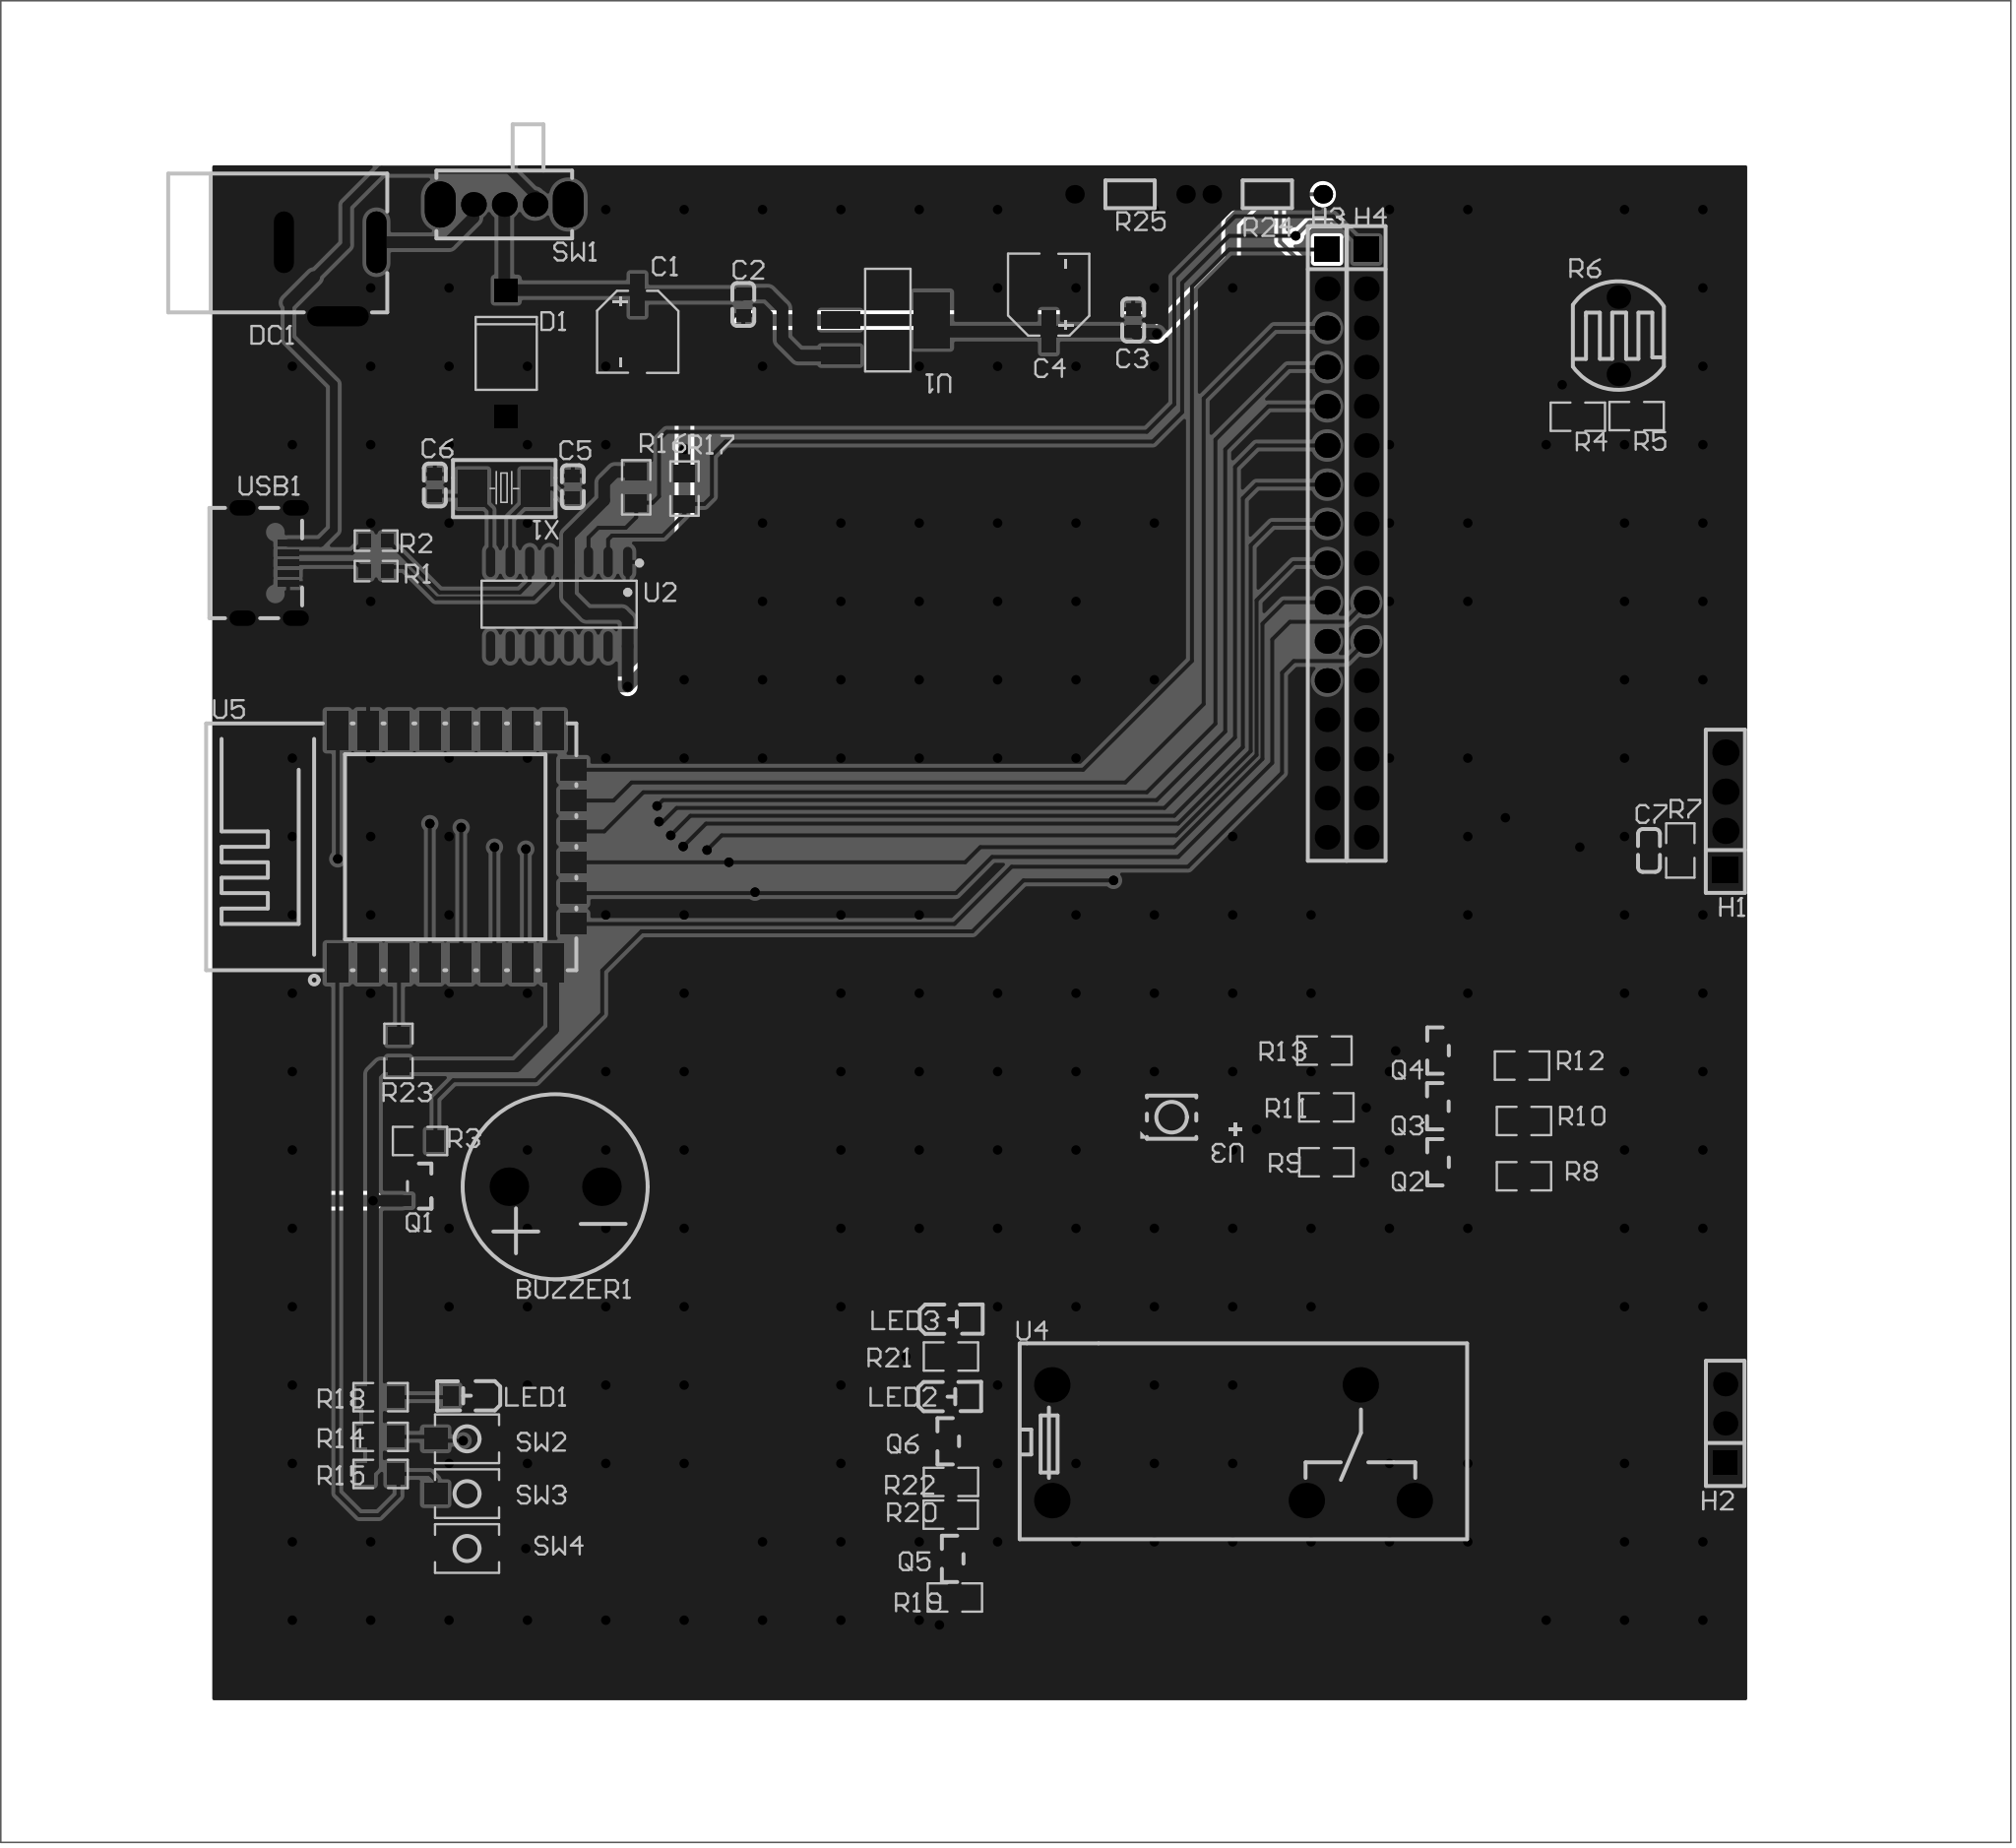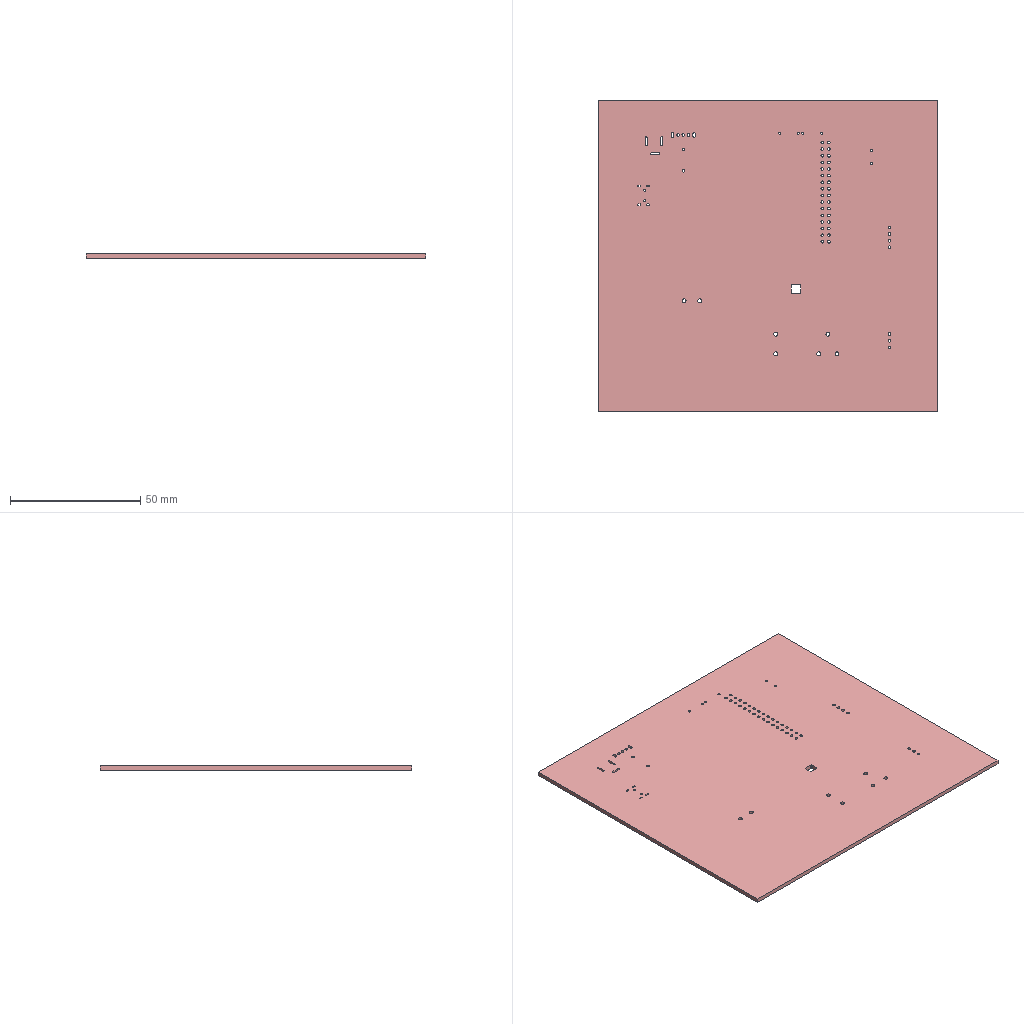Circuit board layout | Altium Designer | box 130.3 x 119.4 x 1.6 mm
Layer stack:
# Altium Designer layer stack of  (unit mm; dielectric type: 0 none, 1 core, 2 prepreg, 3 surface material)
index,name,kind,layer,copper_thickness_mm,dielectric_type,dielectric_thickness_mm,dielectric_material,dielectric_constant
0,Top Paste Mask Layer,other,,,,,,
1,Top Silkscreen Layer,other,,,,,,
2,Top Solder Mask Layer,dielectric,,,3,0.01,,3.3
3,Top Layer,copper,Top Layer,0.035,,,,
4,Dielectric1,dielectric,,,3,1.51,FR4,4.5
5,Bottom Layer,copper,Bottom Layer,0.035,,,,
6,Bottom Solder Mask Layer,dielectric,,,3,0.01,,3.3
7,Bottom Silkscreen Layer,other,,,,,,
8,Bottom Paste Mask Layer,other,,,,,,
# drill layer pairs: low layer,high layer
drill_pair,Top Layer,Bottom Layer
Part placement:
Designator,Comment,Layer,Footprint,Center-X(mm),Center-Y(mm),Rotation
BUZZER1,buzzer,TopLayer,BUZ-TH_BD12.0-P6.00-D0.9-RD,105.788,112.353,180
C1,10uF,TopLayer,C_Ele_SMD_5x5.4mm,111.125,167.767,270
C2,100nF,TopLayer,C0603,117.983,169.545,90
C3,100nF,TopLayer,C0603,143.256,168.529,270
C4,10uF,TopLayer,C_Ele_SMD_5x5.4mm,137.795,170.18,90
C5,22pF,TopLayer,C0603,106.934,157.734,270
C6,22pF,TopLayer,C0603,97.987,157.843,270
C7,100nF,TopLayer,C0603,176.695,134.149,270
D1,SMA_DIODE,TopLayer,SOD-57_BD3.8-L4.6-P9.00-D0.8-RD,102.616,166.37,270
DC1,,TopLayer,DC-2.0,91.204,171.176,180
H1,,TopLayer,HDR-TH_4P-P2.54-V-F,181.648,136.69,90
H2,,TopLayer,HDR-TH_3P-P2.54-V-F,181.637,97.012,90
H3,,TopLayer,HDR-TH_16P-P2.54-V-F,155.829,154.051,270
H4,,TopLayer,HDR-TH_16P-P2.54-V-F,158.369,154.051,270
LED1,,TopLayer,LED_0805,100.126,98.801,180
LED2,,TopLayer,LED_0805,131.423,98.747,0
LED3,,TopLayer,LED_0805,131.522,103.764,0
Q1,,TopLayer,S8550P_SOT,97.113,112.395,180
Q2,,TopLayer,S8050_SOT-23,163.021,113.939,0
Q3,,TopLayer,S8050_SOT-23,163.01,117.571,0
Q4,,TopLayer,S8050_SOT-23,163.021,121.178,0
Q5,,TopLayer,S8050_SOT-23,131.557,88.23,0
Q6,,TopLayer,S8050_SOT-23,131.269,95.85,0
R3,1K,TopLayer,R0805,97.028,115.316,180
R4,10K,TopLayer,R0805,172.083,162.264,0
R5,4.7K,TopLayer,R0805,175.895,162.306,0
R6,GL7528,TopLayer,RES-TH_L7.0-W5.9-P5.00-D0.5,174.711,167.516,0
R7,4.7K,TopLayer,R0805,178.726,134.149,270
R8,1.5K,TopLayer,R0805,168.591,113.031,180
R10,1.5K,TopLayer,R0805,168.591,116.615,180
R12,1.5K,TopLayer,R0805,168.464,120.205,180
R14,10K,TopLayer,R0805,94.472,96.139,0
R15,10K,TopLayer,R0805,94.472,93.734,0
R16,10K,TopLayer,R0805,111.042,157.69,270
R17,10K,TopLayer,R0805,114.173,157.607,270
R18,4.7K,TopLayer,R0805,94.472,98.71,0
R19,1.5K,TopLayer,R0805,131.699,85.725,0
R20,1.5K,TopLayer,R0805,131.43,91.097,0
R21,10K,TopLayer,R0805,131.445,101.346,180
R22,1.5K,TopLayer,R0805,131.445,93.218,0
R23,10K,TopLayer,R0805,95.631,121.158,90
R24,10K,TopLayer,Res_1/8W,151.954,176.686,0
R25,4.7K,TopLayer,Res_1/8W,143.057,176.686,0
SW1,,TopLayer,拨动开关_侧,102.489,176.022,180
SW2,,TopLayer,Key_SMD_3x4x2,100.076,96.012,0
SW3,,TopLayer,Key_SMD_3x4x2,100.076,92.456,0
SW4,,TopLayer,Key_SMD_3x4x2,100.076,88.9,180
U1,AMS1117-3.3,TopLayer,SOT-223-3_L6.5-W3.4-P2.30-LS7.0-BR,127.254,168.529,180
U2,CH340G,TopLayer,SOIC-16_L9.9-W3.9-P1.27-LS6.0-BL,106.045,150.114,180
U3,6028-ZRGBF-SMD-H2,TopLayer,LED-SMD_4P-L3.2-W2.8_ZRGBF-SMD-H2,145.749,116.86,180
U4,SSKD6132,TopLayer,RELAY-TH_G2R-1,149.733,95.758,0
U5,ESP8266,TopLayer,WIFIM-SMD_ESP-12F-ESP8266MOD,99.314,134.387,0
USB1,,TopLayer,USB_Micro,87.249,152.781,270
X1,CRYSTAL,TopLayer,CRYSTAL-SMD_L5.0-W3.2,102.489,157.607,180
R1,27R,TopLayer,R0603,94.18,152.259,180
R2,27R,TopLayer,R0603,94.18,154.232,180
R9,1K,TopLayer,R0805,155.782,113.939,180
R11,1K,TopLayer,R0805,155.782,117.495,180
R13,1K,TopLayer,R0805,155.655,121.178,180
Pad and via stacks:
# Altium Designer via and pad stacks of  (unit mm). Each distinct definition once, with the count of objects using it.
# via: kind,start_layer,end_layer,hole_mm,diameter_mm,mode(0 simple;1 top-mid-bottom;2 full stack),diameter_per_layer,count,example_net
# pad: kind,layer,hole_mm,hole_type(0 round;1 square;2 slot),plating,top_size,top_shape(1 round;2 rect;3 octagon;9 rounded rect),mid_size,bottom_size,mode,footprint,size_per_layer,count,example
pad,Multi-Layer,1.5,0,plated,2.5x2.5,1,2.5x2.5,2.5x2.5,0,BUZ-TH_BD12.0-P6.00-D0.9-RD,,2,BUZZER1.1
pad,Multi-Layer,1,0,plated,1.5x1.5,2,1.5x1.5,1.5x1.5,0,SOD-57_BD3.8-L4.6-P9.00-D0.8-RD,,2,D1.1
pad,Multi-Layer,0.8001,2,plated,4x1.3,1,4x1.3,4x1.3,0,DC-2.0,,3,DC1.2
pad,Multi-Layer,1.1,0,plated,1.7x1.7,2,1.7x1.7,1.7x1.7,0,HDR-TH_4P-P2.54-V-F,,1,H1.1
pad,Multi-Layer,1.1,0,plated,1.7x1.7,1,1.7x1.7,1.7x1.7,0,HDR-TH_4P-P2.54-V-F,,3,H1.2
pad,Multi-Layer,1.02,0,plated,1.575x1.575,1,1.575x1.575,1.575x1.575,0,HDR-TH_3P-P2.54-V-F,,2,H2.3
pad,Multi-Layer,1.02,0,plated,1.575x1.575,2,1.575x1.575,1.575x1.575,0,HDR-TH_3P-P2.54-V-F,,1,H2.1
pad,Multi-Layer,1,0,plated,1.6x1.6,2,1.6x1.6,1.6x1.6,0,HDR-TH_16P-P2.54-V-F,,2,H3.1
pad,Multi-Layer,1,0,plated,1.6x1.6,1,1.6x1.6,1.6x1.6,0,HDR-TH_16P-P2.54-V-F,,30,H3.2
pad,Multi-Layer,0.762,2,plated,1.524x1.524,1,1.524x1.524,1.524x1.524,0,RES-TH_L7.0-W5.9-P5.00-D0.5,,2,R6.2
pad,Multi-Layer,0.8001,0,plated,1.199x1.199,1,1.199x1.199,1.199x1.199,0,Res_1/8W,,4,R24.1
pad,Multi-Layer,1.001,0,plated,1.6x1.6,1,1.6x1.6,1.6x1.6,0,\u00B2\u00A6\u00B6\u00AF\u00BF\u00AA\u00B9\u00D8_\u00B2\u00E0,,3,SW1.1
pad,Multi-Layer,1.001,2,plated,3x1.999,1,3x1.999,3x1.999,0,\u00B2\u00A6\u00B6\u00AF\u00BF\u00AA\u00B9\u00D8_\u00B2\u00E0,,2,SW1.4
pad,Multi-Layer,1.5,0,plated,2.3x2.3,1,2.3x2.3,2.3x2.3,0,RELAY-TH_G2R-1,,5,U4.3
pad,Multi-Layer,0.6,2,plated,1x1.7,1,1x1.7,1x1.7,0,USB_Micro,,4,USB1.6
pad,Top Layer,0,0,plated,2.7x0.91,2,2.7x0.91,2.7x0.91,0,C_Ele_SMD_5x5.4mm,,4,C1.1
pad,Top Layer,0,0,plated,0.8x0.9,2,0.8x0.9,0.8x0.9,0,C0603,,10,C2.2
pad,Top Layer,0,0,plated,1x1.25,2,1x1.25,1x1.25,0,LED_0805,,6,LED1.2
pad,Top Layer,0,0,plated,0.701x1.25,2,0.701x1.25,0.701x1.25,0,S8550P_SOT,,3,Q1.3
pad,Top Layer,0,0,plated,1x0.8,2,1x0.8,1x0.8,0,S8050_SOT-23,,15,Q2.2
pad,Top Layer,0,0,plated,1.133x1.377,2,1.133x1.377,1.133x1.377,0,R0805,,40,R3.2
pad,Top Layer,0,0,plated,1.53x1.36,2,1.53x1.36,1.53x1.36,0,Key_SMD_3x4x2,,6,SW2.1
pad,Top Layer,0,0,plated,2.5x1.1,2,2.5x1.1,2.5x1.1,0,SOT-223-3_L6.5-W3.4-P2.30-LS7.0-BR,,3,U1.1
pad,Top Layer,0,0,plated,2.34x3.6,2,2.34x3.6,2.34x3.6,0,SOT-223-3_L6.5-W3.4-P2.30-LS7.0-BR,,1,U1.4
pad,Top Layer,0,0,plated,0.602x1.971,1,0.602x1.971,0.602x1.971,0,SOIC-16_L9.9-W3.9-P1.27-LS6.0-BL,,16,U2.1
pad,Top Layer,0,0,plated,0.82x1.5,2,0.82x1.5,0.82x1.5,0,LED-SMD_4P-L3.2-W2.8_ZRGBF-SMD-H2,,4,U3.1
pad,Top Layer,0,0,plated,2.5x1.4,2,2.5x1.4,2.5x1.4,0,WIFIM-SMD_ESP-12F-ESP8266MOD,,16,U5.16
pad,Top Layer,0,0,plated,1.7x1.4,2,1.7x1.4,1.7x1.4,0,WIFIM-SMD_ESP-12F-ESP8266MOD,,6,U5.22
pad,Top Layer,0,0,plated,0.4x1.4,2,0.4x1.4,0.4x1.4,0,USB_Micro,,5,USB1.1
pad,Top Layer,0,0,plated,1.9x2.4,2,1.9x2.4,1.9x2.4,0,CRYSTAL-SMD_L5.0-W3.2,,2,X1.2
pad,Top Layer,0,0,plated,0.8065x0.864,2,0.8065x0.864,0.8065x0.864,0,R0603,,4,R1.2
via,Top Layer,Bottom Layer,0.3048,0.61,0,,250,ESP8266_IO16
Copper pours:
name,layer,net,type(0 solid;1 hatched;2 none)
Bottom Layer-GND,Bottom Layer,GND,0
Top Layer-GND,Top Layer,GND,0